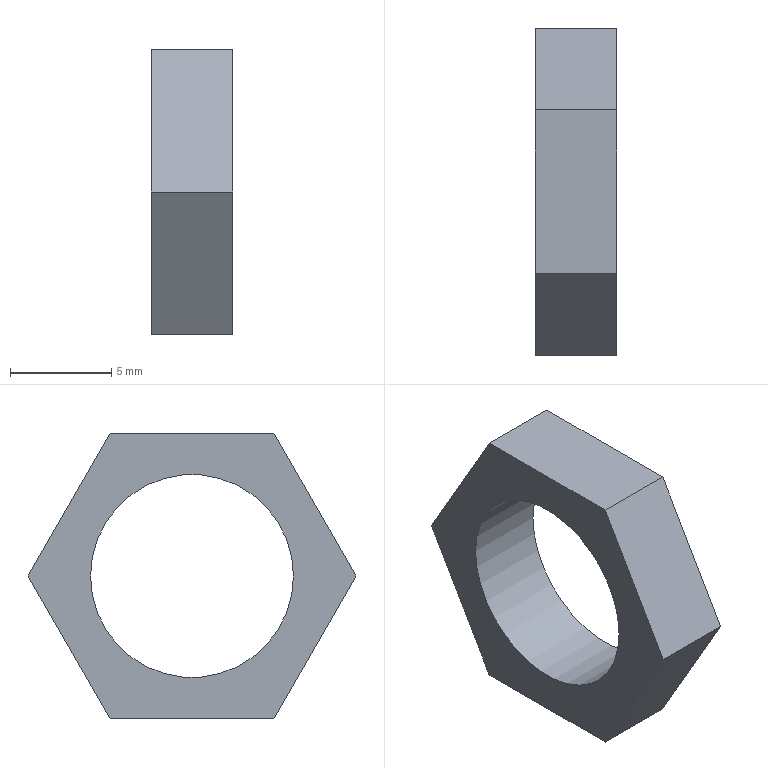Part | STEP file | 1-12.3 | 1 solid | 9 faces | box 4 x 16.166 x 14 mm | volume 364.805 mm3 | plane 8 | cylinder 1 | commonest cylinder face diameters 10 x1
STEP:
#1=CARTESIAN_POINT('',(0.,0.,0.));
#2=DIRECTION('',(0.,0.,1.));
#3=DIRECTION('',(1.,0.,0.));
#4=AXIS2_PLACEMENT_3D('',#1,#2,#3);
#5=CARTESIAN_POINT('',(-2.,8.083,0.));
#6=VERTEX_POINT('',#5);
#7=CARTESIAN_POINT('',(-2.,4.041,7.));
#8=VERTEX_POINT('',#7);
#9=CARTESIAN_POINT('',(-2.,8.083,0.));
#10=DIRECTION('',(0.,-0.5,0.866));
#11=VECTOR('',#10,1.);
#12=LINE('',#9,#11);
#13=CARTESIAN_POINT('',(-2.,0.,1.083));
#14=DIRECTION('',(1.,0.,0.));
#15=DIRECTION('',(0.,1.,0.));
#16=AXIS2_PLACEMENT_3D('',#13,#14,#15);
#17=PLANE('',#16);
#18=CARTESIAN_POINT('',(8.083,-1.083));
#19=DIRECTION('',(-0.5,0.866));
#20=VECTOR('',#19,1.);
#21=LINE('',#18,#20);
#22=(GEOMETRIC_REPRESENTATION_CONTEXT(2)PARAMETRIC_REPRESENTATION_CONTEXT()REPRESENTATION_CONTEXT('',''));
#23=DEFINITIONAL_REPRESENTATION('',(#21),#22);
#24=PCURVE('',#17,#23);
#25=CARTESIAN_POINT('',(0.,6.062,3.5));
#26=DIRECTION('',(0.,0.866,0.5));
#27=DIRECTION('',(0.,-0.5,0.866));
#28=AXIS2_PLACEMENT_3D('',#25,#26,#27);
#29=PLANE('',#28);
#30=CARTESIAN_POINT('',(-4.041,-2.));
#31=DIRECTION('',(1.,0.));
#32=VECTOR('',#31,1.);
#33=LINE('',#30,#32);
#34=(GEOMETRIC_REPRESENTATION_CONTEXT(2)PARAMETRIC_REPRESENTATION_CONTEXT()REPRESENTATION_CONTEXT('',''));
#35=DEFINITIONAL_REPRESENTATION('',(#33),#34);
#36=PCURVE('',#29,#35);
#37=SURFACE_CURVE('',#12,(#24,#36),.PCURVE_S1.);
#38=EDGE_CURVE('',#6,#8,#37,.T.);
#39=ORIENTED_EDGE('',*,*,#38,.T.);
#40=CARTESIAN_POINT('',(-2.,-4.041,7.));
#41=VERTEX_POINT('',#40);
#42=CARTESIAN_POINT('',(-2.,4.041,7.));
#43=DIRECTION('',(0.,-1.,0.));
#44=VECTOR('',#43,1.);
#45=LINE('',#42,#44);
#46=CARTESIAN_POINT('',(4.041,5.917));
#47=DIRECTION('',(-1.,0.));
#48=VECTOR('',#47,1.);
#49=LINE('',#46,#48);
#50=(GEOMETRIC_REPRESENTATION_CONTEXT(2)PARAMETRIC_REPRESENTATION_CONTEXT()REPRESENTATION_CONTEXT('',''));
#51=DEFINITIONAL_REPRESENTATION('',(#49),#50);
#52=PCURVE('',#17,#51);
#53=CARTESIAN_POINT('',(0.,0.,7.));
#54=DIRECTION('',(0.,0.,1.));
#55=DIRECTION('',(0.,-1.,0.));
#56=AXIS2_PLACEMENT_3D('',#53,#54,#55);
#57=PLANE('',#56);
#58=CARTESIAN_POINT('',(-4.041,-2.));
#59=DIRECTION('',(1.,0.));
#60=VECTOR('',#59,1.);
#61=LINE('',#58,#60);
#62=(GEOMETRIC_REPRESENTATION_CONTEXT(2)PARAMETRIC_REPRESENTATION_CONTEXT()REPRESENTATION_CONTEXT('',''));
#63=DEFINITIONAL_REPRESENTATION('',(#61),#62);
#64=PCURVE('',#57,#63);
#65=SURFACE_CURVE('',#45,(#52,#64),.PCURVE_S1.);
#66=EDGE_CURVE('',#8,#41,#65,.T.);
#67=ORIENTED_EDGE('',*,*,#66,.T.);
#68=CARTESIAN_POINT('',(-2.,-8.083,0.));
#69=VERTEX_POINT('',#68);
#70=CARTESIAN_POINT('',(-2.,-4.041,7.));
#71=DIRECTION('',(0.,-0.5,-0.866));
#72=VECTOR('',#71,1.);
#73=LINE('',#70,#72);
#74=CARTESIAN_POINT('',(-4.041,5.917));
#75=DIRECTION('',(-0.5,-0.866));
#76=VECTOR('',#75,1.);
#77=LINE('',#74,#76);
#78=(GEOMETRIC_REPRESENTATION_CONTEXT(2)PARAMETRIC_REPRESENTATION_CONTEXT()REPRESENTATION_CONTEXT('',''));
#79=DEFINITIONAL_REPRESENTATION('',(#77),#78);
#80=PCURVE('',#17,#79);
#81=CARTESIAN_POINT('',(0.,-6.062,3.5));
#82=DIRECTION('',(0.,-0.866,0.5));
#83=DIRECTION('',(0.,-0.5,-0.866));
#84=AXIS2_PLACEMENT_3D('',#81,#82,#83);
#85=PLANE('',#84);
#86=CARTESIAN_POINT('',(-4.041,-2.));
#87=DIRECTION('',(1.,0.));
#88=VECTOR('',#87,1.);
#89=LINE('',#86,#88);
#90=(GEOMETRIC_REPRESENTATION_CONTEXT(2)PARAMETRIC_REPRESENTATION_CONTEXT()REPRESENTATION_CONTEXT('',''));
#91=DEFINITIONAL_REPRESENTATION('',(#89),#90);
#92=PCURVE('',#85,#91);
#93=SURFACE_CURVE('',#73,(#80,#92),.PCURVE_S1.);
#94=EDGE_CURVE('',#41,#69,#93,.T.);
#95=ORIENTED_EDGE('',*,*,#94,.T.);
#96=CARTESIAN_POINT('',(-2.,-4.041,-7.));
#97=VERTEX_POINT('',#96);
#98=CARTESIAN_POINT('',(-2.,-8.083,0.));
#99=DIRECTION('',(0.,0.5,-0.866));
#100=VECTOR('',#99,1.);
#101=LINE('',#98,#100);
#102=CARTESIAN_POINT('',(-8.083,-1.083));
#103=DIRECTION('',(0.5,-0.866));
#104=VECTOR('',#103,1.);
#105=LINE('',#102,#104);
#106=(GEOMETRIC_REPRESENTATION_CONTEXT(2)PARAMETRIC_REPRESENTATION_CONTEXT()REPRESENTATION_CONTEXT('',''));
#107=DEFINITIONAL_REPRESENTATION('',(#105),#106);
#108=PCURVE('',#17,#107);
#109=CARTESIAN_POINT('',(0.,-6.062,-3.5));
#110=DIRECTION('',(0.,-0.866,-0.5));
#111=DIRECTION('',(0.,0.5,-0.866));
#112=AXIS2_PLACEMENT_3D('',#109,#110,#111);
#113=PLANE('',#112);
#114=CARTESIAN_POINT('',(-4.041,-2.));
#115=DIRECTION('',(1.,0.));
#116=VECTOR('',#115,1.);
#117=LINE('',#114,#116);
#118=(GEOMETRIC_REPRESENTATION_CONTEXT(2)PARAMETRIC_REPRESENTATION_CONTEXT()REPRESENTATION_CONTEXT('',''));
#119=DEFINITIONAL_REPRESENTATION('',(#117),#118);
#120=PCURVE('',#113,#119);
#121=SURFACE_CURVE('',#101,(#108,#120),.PCURVE_S1.);
#122=EDGE_CURVE('',#69,#97,#121,.T.);
#123=ORIENTED_EDGE('',*,*,#122,.T.);
#124=CARTESIAN_POINT('',(-2.,4.041,-7.));
#125=VERTEX_POINT('',#124);
#126=CARTESIAN_POINT('',(-2.,-4.041,-7.));
#127=DIRECTION('',(0.,1.,0.));
#128=VECTOR('',#127,1.);
#129=LINE('',#126,#128);
#130=CARTESIAN_POINT('',(-4.041,-8.083));
#131=DIRECTION('',(1.,0.));
#132=VECTOR('',#131,1.);
#133=LINE('',#130,#132);
#134=(GEOMETRIC_REPRESENTATION_CONTEXT(2)PARAMETRIC_REPRESENTATION_CONTEXT()REPRESENTATION_CONTEXT('',''));
#135=DEFINITIONAL_REPRESENTATION('',(#133),#134);
#136=PCURVE('',#17,#135);
#137=CARTESIAN_POINT('',(0.,0.,-7.));
#138=DIRECTION('',(0.,0.,-1.));
#139=DIRECTION('',(0.,1.,0.));
#140=AXIS2_PLACEMENT_3D('',#137,#138,#139);
#141=PLANE('',#140);
#142=CARTESIAN_POINT('',(-4.041,-2.));
#143=DIRECTION('',(1.,0.));
#144=VECTOR('',#143,1.);
#145=LINE('',#142,#144);
#146=(GEOMETRIC_REPRESENTATION_CONTEXT(2)PARAMETRIC_REPRESENTATION_CONTEXT()REPRESENTATION_CONTEXT('',''));
#147=DEFINITIONAL_REPRESENTATION('',(#145),#146);
#148=PCURVE('',#141,#147);
#149=SURFACE_CURVE('',#129,(#136,#148),.PCURVE_S1.);
#150=EDGE_CURVE('',#97,#125,#149,.T.);
#151=ORIENTED_EDGE('',*,*,#150,.T.);
#152=CARTESIAN_POINT('',(-2.,4.041,-7.));
#153=DIRECTION('',(0.,0.5,0.866));
#154=VECTOR('',#153,1.);
#155=LINE('',#152,#154);
#156=CARTESIAN_POINT('',(4.041,-8.083));
#157=DIRECTION('',(0.5,0.866));
#158=VECTOR('',#157,1.);
#159=LINE('',#156,#158);
#160=(GEOMETRIC_REPRESENTATION_CONTEXT(2)PARAMETRIC_REPRESENTATION_CONTEXT()REPRESENTATION_CONTEXT('',''));
#161=DEFINITIONAL_REPRESENTATION('',(#159),#160);
#162=PCURVE('',#17,#161);
#163=CARTESIAN_POINT('',(0.,6.062,-3.5));
#164=DIRECTION('',(0.,0.866,-0.5));
#165=DIRECTION('',(0.,0.5,0.866));
#166=AXIS2_PLACEMENT_3D('',#163,#164,#165);
#167=PLANE('',#166);
#168=CARTESIAN_POINT('',(-4.041,-2.));
#169=DIRECTION('',(1.,0.));
#170=VECTOR('',#169,1.);
#171=LINE('',#168,#170);
#172=(GEOMETRIC_REPRESENTATION_CONTEXT(2)PARAMETRIC_REPRESENTATION_CONTEXT()REPRESENTATION_CONTEXT('',''));
#173=DEFINITIONAL_REPRESENTATION('',(#171),#172);
#174=PCURVE('',#167,#173);
#175=SURFACE_CURVE('',#155,(#162,#174),.PCURVE_S1.);
#176=EDGE_CURVE('',#125,#6,#175,.T.);
#177=ORIENTED_EDGE('',*,*,#176,.T.);
#178=EDGE_LOOP('',(#39,#67,#95,#123,#151,#177));
#179=FACE_BOUND('',#178,.F.);
#180=CARTESIAN_POINT('',(-2.,5.,0.));
#181=VERTEX_POINT('',#180);
#182=CARTESIAN_POINT('',(-2.,0.,0.));
#183=DIRECTION('',(-1.,0.,0.));
#184=DIRECTION('',(0.,1.,0.));
#185=AXIS2_PLACEMENT_3D('',#182,#183,#184);
#186=CIRCLE('',#185,5.);
#187=CARTESIAN_POINT('',(5.,-1.083));
#188=CARTESIAN_POINT('',(5.,-9.743));
#189=CARTESIAN_POINT('',(-2.5,-5.413));
#190=CARTESIAN_POINT('',(-10.,-1.083));
#191=CARTESIAN_POINT('',(-2.5,3.247));
#192=CARTESIAN_POINT('',(5.,7.577));
#193=CARTESIAN_POINT('',(5.,-1.083));
#194=(BOUNDED_CURVE()B_SPLINE_CURVE(2,(#187,#188,#189,#190,#191,#192,#193),.UNSPECIFIED.,.T.,.F.)B_SPLINE_CURVE_WITH_KNOTS((1,2,2,2,2,1),(-2.094,0.,2.094,4.189,6.283,8.378),.UNSPECIFIED.)CURVE()GEOMETRIC_REPRESENTATION_ITEM()RATIONAL_B_SPLINE_CURVE((1.,0.5,1.,0.5,1.,0.5,1.))REPRESENTATION_ITEM(''));
#195=(GEOMETRIC_REPRESENTATION_CONTEXT(2)PARAMETRIC_REPRESENTATION_CONTEXT()REPRESENTATION_CONTEXT('',''));
#196=DEFINITIONAL_REPRESENTATION('',(#194),#195);
#197=PCURVE('',#17,#196);
#198=CARTESIAN_POINT('',(-2.,0.,0.));
#199=DIRECTION('',(1.,0.,0.));
#200=DIRECTION('',(0.,1.,0.));
#201=AXIS2_PLACEMENT_3D('',#198,#199,#200);
#202=CYLINDRICAL_SURFACE('',#201,5.);
#203=CARTESIAN_POINT('',(6.283,0.));
#204=DIRECTION('',(-1.,0.));
#205=VECTOR('',#204,1.);
#206=LINE('',#203,#205);
#207=(GEOMETRIC_REPRESENTATION_CONTEXT(2)PARAMETRIC_REPRESENTATION_CONTEXT()REPRESENTATION_CONTEXT('',''));
#208=DEFINITIONAL_REPRESENTATION('',(#206),#207);
#209=PCURVE('',#202,#208);
#210=SURFACE_CURVE('',#186,(#197,#209),.PCURVE_S1.);
#211=EDGE_CURVE('',#181,#181,#210,.T.);
#212=ORIENTED_EDGE('',*,*,#211,.T.);
#213=EDGE_LOOP('',(#212));
#214=FACE_BOUND('',#213,.F.);
#215=ADVANCED_FACE('',(#179,#214),#17,.F.);
#216=CARTESIAN_POINT('',(2.,8.083,0.));
#217=VERTEX_POINT('',#216);
#218=CARTESIAN_POINT('',(2.,4.041,7.));
#219=VERTEX_POINT('',#218);
#220=CARTESIAN_POINT('',(2.,8.083,0.));
#221=DIRECTION('',(0.,-0.5,0.866));
#222=VECTOR('',#221,1.);
#223=LINE('',#220,#222);
#224=CARTESIAN_POINT('',(2.,0.,1.083));
#225=DIRECTION('',(1.,0.,0.));
#226=DIRECTION('',(0.,1.,0.));
#227=AXIS2_PLACEMENT_3D('',#224,#225,#226);
#228=PLANE('',#227);
#229=CARTESIAN_POINT('',(8.083,-1.083));
#230=DIRECTION('',(-0.5,0.866));
#231=VECTOR('',#230,1.);
#232=LINE('',#229,#231);
#233=(GEOMETRIC_REPRESENTATION_CONTEXT(2)PARAMETRIC_REPRESENTATION_CONTEXT()REPRESENTATION_CONTEXT('',''));
#234=DEFINITIONAL_REPRESENTATION('',(#232),#233);
#235=PCURVE('',#228,#234);
#236=CARTESIAN_POINT('',(-4.041,2.));
#237=DIRECTION('',(1.,0.));
#238=VECTOR('',#237,1.);
#239=LINE('',#236,#238);
#240=(GEOMETRIC_REPRESENTATION_CONTEXT(2)PARAMETRIC_REPRESENTATION_CONTEXT()REPRESENTATION_CONTEXT('',''));
#241=DEFINITIONAL_REPRESENTATION('',(#239),#240);
#242=PCURVE('',#29,#241);
#243=SURFACE_CURVE('',#223,(#235,#242),.PCURVE_S1.);
#244=EDGE_CURVE('',#217,#219,#243,.T.);
#245=ORIENTED_EDGE('',*,*,#244,.T.);
#246=CARTESIAN_POINT('',(2.,-4.041,7.));
#247=VERTEX_POINT('',#246);
#248=CARTESIAN_POINT('',(2.,4.041,7.));
#249=DIRECTION('',(0.,-1.,0.));
#250=VECTOR('',#249,1.);
#251=LINE('',#248,#250);
#252=CARTESIAN_POINT('',(4.041,5.917));
#253=DIRECTION('',(-1.,0.));
#254=VECTOR('',#253,1.);
#255=LINE('',#252,#254);
#256=(GEOMETRIC_REPRESENTATION_CONTEXT(2)PARAMETRIC_REPRESENTATION_CONTEXT()REPRESENTATION_CONTEXT('',''));
#257=DEFINITIONAL_REPRESENTATION('',(#255),#256);
#258=PCURVE('',#228,#257);
#259=CARTESIAN_POINT('',(-4.041,2.));
#260=DIRECTION('',(1.,0.));
#261=VECTOR('',#260,1.);
#262=LINE('',#259,#261);
#263=(GEOMETRIC_REPRESENTATION_CONTEXT(2)PARAMETRIC_REPRESENTATION_CONTEXT()REPRESENTATION_CONTEXT('',''));
#264=DEFINITIONAL_REPRESENTATION('',(#262),#263);
#265=PCURVE('',#57,#264);
#266=SURFACE_CURVE('',#251,(#258,#265),.PCURVE_S1.);
#267=EDGE_CURVE('',#219,#247,#266,.T.);
#268=ORIENTED_EDGE('',*,*,#267,.T.);
#269=CARTESIAN_POINT('',(2.,-8.083,0.));
#270=VERTEX_POINT('',#269);
#271=CARTESIAN_POINT('',(2.,-4.041,7.));
#272=DIRECTION('',(0.,-0.5,-0.866));
#273=VECTOR('',#272,1.);
#274=LINE('',#271,#273);
#275=CARTESIAN_POINT('',(-4.041,5.917));
#276=DIRECTION('',(-0.5,-0.866));
#277=VECTOR('',#276,1.);
#278=LINE('',#275,#277);
#279=(GEOMETRIC_REPRESENTATION_CONTEXT(2)PARAMETRIC_REPRESENTATION_CONTEXT()REPRESENTATION_CONTEXT('',''));
#280=DEFINITIONAL_REPRESENTATION('',(#278),#279);
#281=PCURVE('',#228,#280);
#282=CARTESIAN_POINT('',(-4.041,2.));
#283=DIRECTION('',(1.,0.));
#284=VECTOR('',#283,1.);
#285=LINE('',#282,#284);
#286=(GEOMETRIC_REPRESENTATION_CONTEXT(2)PARAMETRIC_REPRESENTATION_CONTEXT()REPRESENTATION_CONTEXT('',''));
#287=DEFINITIONAL_REPRESENTATION('',(#285),#286);
#288=PCURVE('',#85,#287);
#289=SURFACE_CURVE('',#274,(#281,#288),.PCURVE_S1.);
#290=EDGE_CURVE('',#247,#270,#289,.T.);
#291=ORIENTED_EDGE('',*,*,#290,.T.);
#292=CARTESIAN_POINT('',(2.,-4.041,-7.));
#293=VERTEX_POINT('',#292);
#294=CARTESIAN_POINT('',(2.,-8.083,0.));
#295=DIRECTION('',(0.,0.5,-0.866));
#296=VECTOR('',#295,1.);
#297=LINE('',#294,#296);
#298=CARTESIAN_POINT('',(-8.083,-1.083));
#299=DIRECTION('',(0.5,-0.866));
#300=VECTOR('',#299,1.);
#301=LINE('',#298,#300);
#302=(GEOMETRIC_REPRESENTATION_CONTEXT(2)PARAMETRIC_REPRESENTATION_CONTEXT()REPRESENTATION_CONTEXT('',''));
#303=DEFINITIONAL_REPRESENTATION('',(#301),#302);
#304=PCURVE('',#228,#303);
#305=CARTESIAN_POINT('',(-4.041,2.));
#306=DIRECTION('',(1.,0.));
#307=VECTOR('',#306,1.);
#308=LINE('',#305,#307);
#309=(GEOMETRIC_REPRESENTATION_CONTEXT(2)PARAMETRIC_REPRESENTATION_CONTEXT()REPRESENTATION_CONTEXT('',''));
#310=DEFINITIONAL_REPRESENTATION('',(#308),#309);
#311=PCURVE('',#113,#310);
#312=SURFACE_CURVE('',#297,(#304,#311),.PCURVE_S1.);
#313=EDGE_CURVE('',#270,#293,#312,.T.);
#314=ORIENTED_EDGE('',*,*,#313,.T.);
#315=CARTESIAN_POINT('',(2.,4.041,-7.));
#316=VERTEX_POINT('',#315);
#317=CARTESIAN_POINT('',(2.,-4.041,-7.));
#318=DIRECTION('',(0.,1.,0.));
#319=VECTOR('',#318,1.);
#320=LINE('',#317,#319);
#321=CARTESIAN_POINT('',(-4.041,-8.083));
#322=DIRECTION('',(1.,0.));
#323=VECTOR('',#322,1.);
#324=LINE('',#321,#323);
#325=(GEOMETRIC_REPRESENTATION_CONTEXT(2)PARAMETRIC_REPRESENTATION_CONTEXT()REPRESENTATION_CONTEXT('',''));
#326=DEFINITIONAL_REPRESENTATION('',(#324),#325);
#327=PCURVE('',#228,#326);
#328=CARTESIAN_POINT('',(-4.041,2.));
#329=DIRECTION('',(1.,0.));
#330=VECTOR('',#329,1.);
#331=LINE('',#328,#330);
#332=(GEOMETRIC_REPRESENTATION_CONTEXT(2)PARAMETRIC_REPRESENTATION_CONTEXT()REPRESENTATION_CONTEXT('',''));
#333=DEFINITIONAL_REPRESENTATION('',(#331),#332);
#334=PCURVE('',#141,#333);
#335=SURFACE_CURVE('',#320,(#327,#334),.PCURVE_S1.);
#336=EDGE_CURVE('',#293,#316,#335,.T.);
#337=ORIENTED_EDGE('',*,*,#336,.T.);
#338=CARTESIAN_POINT('',(2.,4.041,-7.));
#339=DIRECTION('',(0.,0.5,0.866));
#340=VECTOR('',#339,1.);
#341=LINE('',#338,#340);
#342=CARTESIAN_POINT('',(4.041,-8.083));
#343=DIRECTION('',(0.5,0.866));
#344=VECTOR('',#343,1.);
#345=LINE('',#342,#344);
#346=(GEOMETRIC_REPRESENTATION_CONTEXT(2)PARAMETRIC_REPRESENTATION_CONTEXT()REPRESENTATION_CONTEXT('',''));
#347=DEFINITIONAL_REPRESENTATION('',(#345),#346);
#348=PCURVE('',#228,#347);
#349=CARTESIAN_POINT('',(-4.041,2.));
#350=DIRECTION('',(1.,0.));
#351=VECTOR('',#350,1.);
#352=LINE('',#349,#351);
#353=(GEOMETRIC_REPRESENTATION_CONTEXT(2)PARAMETRIC_REPRESENTATION_CONTEXT()REPRESENTATION_CONTEXT('',''));
#354=DEFINITIONAL_REPRESENTATION('',(#352),#353);
#355=PCURVE('',#167,#354);
#356=SURFACE_CURVE('',#341,(#348,#355),.PCURVE_S1.);
#357=EDGE_CURVE('',#316,#217,#356,.T.);
#358=ORIENTED_EDGE('',*,*,#357,.T.);
#359=EDGE_LOOP('',(#245,#268,#291,#314,#337,#358));
#360=FACE_BOUND('',#359,.T.);
#361=CARTESIAN_POINT('',(2.,5.,0.));
#362=VERTEX_POINT('',#361);
#363=CARTESIAN_POINT('',(2.,0.,0.));
#364=DIRECTION('',(-1.,0.,0.));
#365=DIRECTION('',(0.,1.,0.));
#366=AXIS2_PLACEMENT_3D('',#363,#364,#365);
#367=CIRCLE('',#366,5.);
#368=CARTESIAN_POINT('',(5.,-1.083));
#369=CARTESIAN_POINT('',(5.,-9.743));
#370=CARTESIAN_POINT('',(-2.5,-5.413));
#371=CARTESIAN_POINT('',(-10.,-1.083));
#372=CARTESIAN_POINT('',(-2.5,3.247));
#373=CARTESIAN_POINT('',(5.,7.577));
#374=CARTESIAN_POINT('',(5.,-1.083));
#375=(BOUNDED_CURVE()B_SPLINE_CURVE(2,(#368,#369,#370,#371,#372,#373,#374),.UNSPECIFIED.,.T.,.F.)B_SPLINE_CURVE_WITH_KNOTS((1,2,2,2,2,1),(-2.094,0.,2.094,4.189,6.283,8.378),.UNSPECIFIED.)CURVE()GEOMETRIC_REPRESENTATION_ITEM()RATIONAL_B_SPLINE_CURVE((1.,0.5,1.,0.5,1.,0.5,1.))REPRESENTATION_ITEM(''));
#376=(GEOMETRIC_REPRESENTATION_CONTEXT(2)PARAMETRIC_REPRESENTATION_CONTEXT()REPRESENTATION_CONTEXT('',''));
#377=DEFINITIONAL_REPRESENTATION('',(#375),#376);
#378=PCURVE('',#228,#377);
#379=CARTESIAN_POINT('',(6.283,4.));
#380=DIRECTION('',(-1.,0.));
#381=VECTOR('',#380,1.);
#382=LINE('',#379,#381);
#383=(GEOMETRIC_REPRESENTATION_CONTEXT(2)PARAMETRIC_REPRESENTATION_CONTEXT()REPRESENTATION_CONTEXT('',''));
#384=DEFINITIONAL_REPRESENTATION('',(#382),#383);
#385=PCURVE('',#202,#384);
#386=SURFACE_CURVE('',#367,(#378,#385),.PCURVE_S1.);
#387=EDGE_CURVE('',#362,#362,#386,.T.);
#388=ORIENTED_EDGE('',*,*,#387,.T.);
#389=EDGE_LOOP('',(#388));
#390=FACE_BOUND('',#389,.T.);
#391=ADVANCED_FACE('',(#360,#390),#228,.T.);
#392=ORIENTED_EDGE('',*,*,#38,.T.);
#393=CARTESIAN_POINT('',(-2.,4.041,7.));
#394=DIRECTION('',(1.,0.,0.));
#395=VECTOR('',#394,1.);
#396=LINE('',#393,#395);
#397=CARTESIAN_POINT('',(4.041,-2.));
#398=DIRECTION('',(0.,1.));
#399=VECTOR('',#398,1.);
#400=LINE('',#397,#399);
#401=(GEOMETRIC_REPRESENTATION_CONTEXT(2)PARAMETRIC_REPRESENTATION_CONTEXT()REPRESENTATION_CONTEXT('',''));
#402=DEFINITIONAL_REPRESENTATION('',(#400),#401);
#403=PCURVE('',#29,#402);
#404=CARTESIAN_POINT('',(-4.041,-2.));
#405=DIRECTION('',(0.,1.));
#406=VECTOR('',#405,1.);
#407=LINE('',#404,#406);
#408=(GEOMETRIC_REPRESENTATION_CONTEXT(2)PARAMETRIC_REPRESENTATION_CONTEXT()REPRESENTATION_CONTEXT('',''));
#409=DEFINITIONAL_REPRESENTATION('',(#407),#408);
#410=PCURVE('',#57,#409);
#411=SURFACE_CURVE('',#396,(#403,#410),.PCURVE_S1.);
#412=EDGE_CURVE('',#8,#219,#411,.T.);
#413=ORIENTED_EDGE('',*,*,#412,.T.);
#414=ORIENTED_EDGE('',*,*,#244,.F.);
#415=CARTESIAN_POINT('',(-2.,8.083,0.));
#416=DIRECTION('',(1.,0.,0.));
#417=VECTOR('',#416,1.);
#418=LINE('',#415,#417);
#419=CARTESIAN_POINT('',(-4.041,-2.));
#420=DIRECTION('',(0.,1.));
#421=VECTOR('',#420,1.);
#422=LINE('',#419,#421);
#423=(GEOMETRIC_REPRESENTATION_CONTEXT(2)PARAMETRIC_REPRESENTATION_CONTEXT()REPRESENTATION_CONTEXT('',''));
#424=DEFINITIONAL_REPRESENTATION('',(#422),#423);
#425=PCURVE('',#29,#424);
#426=CARTESIAN_POINT('',(4.041,-2.));
#427=DIRECTION('',(0.,1.));
#428=VECTOR('',#427,1.);
#429=LINE('',#426,#428);
#430=(GEOMETRIC_REPRESENTATION_CONTEXT(2)PARAMETRIC_REPRESENTATION_CONTEXT()REPRESENTATION_CONTEXT('',''));
#431=DEFINITIONAL_REPRESENTATION('',(#429),#430);
#432=PCURVE('',#167,#431);
#433=SURFACE_CURVE('',#418,(#425,#432),.PCURVE_S1.);
#434=EDGE_CURVE('',#6,#217,#433,.T.);
#435=ORIENTED_EDGE('',*,*,#434,.F.);
#436=EDGE_LOOP('',(#392,#413,#414,#435));
#437=FACE_BOUND('',#436,.T.);
#438=ADVANCED_FACE('',(#437),#29,.T.);
#439=ORIENTED_EDGE('',*,*,#66,.T.);
#440=CARTESIAN_POINT('',(-2.,-4.041,7.));
#441=DIRECTION('',(1.,0.,0.));
#442=VECTOR('',#441,1.);
#443=LINE('',#440,#442);
#444=CARTESIAN_POINT('',(4.041,-2.));
#445=DIRECTION('',(0.,1.));
#446=VECTOR('',#445,1.);
#447=LINE('',#444,#446);
#448=(GEOMETRIC_REPRESENTATION_CONTEXT(2)PARAMETRIC_REPRESENTATION_CONTEXT()REPRESENTATION_CONTEXT('',''));
#449=DEFINITIONAL_REPRESENTATION('',(#447),#448);
#450=PCURVE('',#57,#449);
#451=CARTESIAN_POINT('',(-4.041,-2.));
#452=DIRECTION('',(0.,1.));
#453=VECTOR('',#452,1.);
#454=LINE('',#451,#453);
#455=(GEOMETRIC_REPRESENTATION_CONTEXT(2)PARAMETRIC_REPRESENTATION_CONTEXT()REPRESENTATION_CONTEXT('',''));
#456=DEFINITIONAL_REPRESENTATION('',(#454),#455);
#457=PCURVE('',#85,#456);
#458=SURFACE_CURVE('',#443,(#450,#457),.PCURVE_S1.);
#459=EDGE_CURVE('',#41,#247,#458,.T.);
#460=ORIENTED_EDGE('',*,*,#459,.T.);
#461=ORIENTED_EDGE('',*,*,#267,.F.);
#462=ORIENTED_EDGE('',*,*,#412,.F.);
#463=EDGE_LOOP('',(#439,#460,#461,#462));
#464=FACE_BOUND('',#463,.T.);
#465=ADVANCED_FACE('',(#464),#57,.T.);
#466=ORIENTED_EDGE('',*,*,#94,.T.);
#467=CARTESIAN_POINT('',(-2.,-8.083,0.));
#468=DIRECTION('',(1.,0.,0.));
#469=VECTOR('',#468,1.);
#470=LINE('',#467,#469);
#471=CARTESIAN_POINT('',(4.041,-2.));
#472=DIRECTION('',(0.,1.));
#473=VECTOR('',#472,1.);
#474=LINE('',#471,#473);
#475=(GEOMETRIC_REPRESENTATION_CONTEXT(2)PARAMETRIC_REPRESENTATION_CONTEXT()REPRESENTATION_CONTEXT('',''));
#476=DEFINITIONAL_REPRESENTATION('',(#474),#475);
#477=PCURVE('',#85,#476);
#478=CARTESIAN_POINT('',(-4.041,-2.));
#479=DIRECTION('',(0.,1.));
#480=VECTOR('',#479,1.);
#481=LINE('',#478,#480);
#482=(GEOMETRIC_REPRESENTATION_CONTEXT(2)PARAMETRIC_REPRESENTATION_CONTEXT()REPRESENTATION_CONTEXT('',''));
#483=DEFINITIONAL_REPRESENTATION('',(#481),#482);
#484=PCURVE('',#113,#483);
#485=SURFACE_CURVE('',#470,(#477,#484),.PCURVE_S1.);
#486=EDGE_CURVE('',#69,#270,#485,.T.);
#487=ORIENTED_EDGE('',*,*,#486,.T.);
#488=ORIENTED_EDGE('',*,*,#290,.F.);
#489=ORIENTED_EDGE('',*,*,#459,.F.);
#490=EDGE_LOOP('',(#466,#487,#488,#489));
#491=FACE_BOUND('',#490,.T.);
#492=ADVANCED_FACE('',(#491),#85,.T.);
#493=ORIENTED_EDGE('',*,*,#122,.T.);
#494=CARTESIAN_POINT('',(-2.,-4.041,-7.));
#495=DIRECTION('',(1.,0.,0.));
#496=VECTOR('',#495,1.);
#497=LINE('',#494,#496);
#498=CARTESIAN_POINT('',(4.041,-2.));
#499=DIRECTION('',(0.,1.));
#500=VECTOR('',#499,1.);
#501=LINE('',#498,#500);
#502=(GEOMETRIC_REPRESENTATION_CONTEXT(2)PARAMETRIC_REPRESENTATION_CONTEXT()REPRESENTATION_CONTEXT('',''));
#503=DEFINITIONAL_REPRESENTATION('',(#501),#502);
#504=PCURVE('',#113,#503);
#505=CARTESIAN_POINT('',(-4.041,-2.));
#506=DIRECTION('',(0.,1.));
#507=VECTOR('',#506,1.);
#508=LINE('',#505,#507);
#509=(GEOMETRIC_REPRESENTATION_CONTEXT(2)PARAMETRIC_REPRESENTATION_CONTEXT()REPRESENTATION_CONTEXT('',''));
#510=DEFINITIONAL_REPRESENTATION('',(#508),#509);
#511=PCURVE('',#141,#510);
#512=SURFACE_CURVE('',#497,(#504,#511),.PCURVE_S1.);
#513=EDGE_CURVE('',#97,#293,#512,.T.);
#514=ORIENTED_EDGE('',*,*,#513,.T.);
#515=ORIENTED_EDGE('',*,*,#313,.F.);
#516=ORIENTED_EDGE('',*,*,#486,.F.);
#517=EDGE_LOOP('',(#493,#514,#515,#516));
#518=FACE_BOUND('',#517,.T.);
#519=ADVANCED_FACE('',(#518),#113,.T.);
#520=ORIENTED_EDGE('',*,*,#150,.T.);
#521=CARTESIAN_POINT('',(-2.,4.041,-7.));
#522=DIRECTION('',(1.,0.,0.));
#523=VECTOR('',#522,1.);
#524=LINE('',#521,#523);
#525=CARTESIAN_POINT('',(4.041,-2.));
#526=DIRECTION('',(0.,1.));
#527=VECTOR('',#526,1.);
#528=LINE('',#525,#527);
#529=(GEOMETRIC_REPRESENTATION_CONTEXT(2)PARAMETRIC_REPRESENTATION_CONTEXT()REPRESENTATION_CONTEXT('',''));
#530=DEFINITIONAL_REPRESENTATION('',(#528),#529);
#531=PCURVE('',#141,#530);
#532=CARTESIAN_POINT('',(-4.041,-2.));
#533=DIRECTION('',(0.,1.));
#534=VECTOR('',#533,1.);
#535=LINE('',#532,#534);
#536=(GEOMETRIC_REPRESENTATION_CONTEXT(2)PARAMETRIC_REPRESENTATION_CONTEXT()REPRESENTATION_CONTEXT('',''));
#537=DEFINITIONAL_REPRESENTATION('',(#535),#536);
#538=PCURVE('',#167,#537);
#539=SURFACE_CURVE('',#524,(#531,#538),.PCURVE_S1.);
#540=EDGE_CURVE('',#125,#316,#539,.T.);
#541=ORIENTED_EDGE('',*,*,#540,.T.);
#542=ORIENTED_EDGE('',*,*,#336,.F.);
#543=ORIENTED_EDGE('',*,*,#513,.F.);
#544=EDGE_LOOP('',(#520,#541,#542,#543));
#545=FACE_BOUND('',#544,.T.);
#546=ADVANCED_FACE('',(#545),#141,.T.);
#547=ORIENTED_EDGE('',*,*,#176,.T.);
#548=ORIENTED_EDGE('',*,*,#434,.T.);
#549=ORIENTED_EDGE('',*,*,#357,.F.);
#550=ORIENTED_EDGE('',*,*,#540,.F.);
#551=EDGE_LOOP('',(#547,#548,#549,#550));
#552=FACE_BOUND('',#551,.T.);
#553=ADVANCED_FACE('',(#552),#167,.T.);
#554=CARTESIAN_POINT('',(-2.,5.,0.));
#555=DIRECTION('',(1.,0.,0.));
#556=VECTOR('',#555,1.);
#557=LINE('',#554,#556);
#558=CARTESIAN_POINT('',(6.283,0.));
#559=DIRECTION('',(0.,1.));
#560=VECTOR('',#559,1.);
#561=LINE('',#558,#560);
#562=(GEOMETRIC_REPRESENTATION_CONTEXT(2)PARAMETRIC_REPRESENTATION_CONTEXT()REPRESENTATION_CONTEXT('',''));
#563=DEFINITIONAL_REPRESENTATION('',(#561),#562);
#564=PCURVE('',#202,#563);
#565=CARTESIAN_POINT('',(0.,0.));
#566=DIRECTION('',(0.,1.));
#567=VECTOR('',#566,1.);
#568=LINE('',#565,#567);
#569=(GEOMETRIC_REPRESENTATION_CONTEXT(2)PARAMETRIC_REPRESENTATION_CONTEXT()REPRESENTATION_CONTEXT('',''));
#570=DEFINITIONAL_REPRESENTATION('',(#568),#569);
#571=PCURVE('',#202,#570);
#572=SEAM_CURVE('',#557,(#564,#571),.PCURVE_S1.);
#573=EDGE_CURVE('',#181,#362,#572,.T.);
#574=ORIENTED_EDGE('',*,*,#573,.T.);
#575=ORIENTED_EDGE('',*,*,#387,.T.);
#576=ORIENTED_EDGE('',*,*,#573,.F.);
#577=ORIENTED_EDGE('',*,*,#211,.F.);
#578=EDGE_LOOP('',(#574,#575,#576,#577));
#579=FACE_BOUND('',#578,.F.);
#580=ADVANCED_FACE('',(#579),#202,.F.);
#581=CLOSED_SHELL('',(#215,#391,#438,#465,#492,#519,#546,#553,#580));
#582=MANIFOLD_SOLID_BREP('',#581);
#583=(LENGTH_UNIT()NAMED_UNIT(*)SI_UNIT(.MILLI.,.METRE.));
#584=UNCERTAINTY_MEASURE_WITH_UNIT(LENGTH_MEASURE(0.0000001),#583,'','');
#585=(NAMED_UNIT(*)PLANE_ANGLE_UNIT()SI_UNIT($,.RADIAN.));
#586=(NAMED_UNIT(*)SI_UNIT($,.STERADIAN.)SOLID_ANGLE_UNIT());
#587=(GEOMETRIC_REPRESENTATION_CONTEXT(3)GLOBAL_UNCERTAINTY_ASSIGNED_CONTEXT((#584))GLOBAL_UNIT_ASSIGNED_CONTEXT((#583,#585,#586))REPRESENTATION_CONTEXT('',''));
#588=ADVANCED_BREP_SHAPE_REPRESENTATION('',(#4,#582),#587);